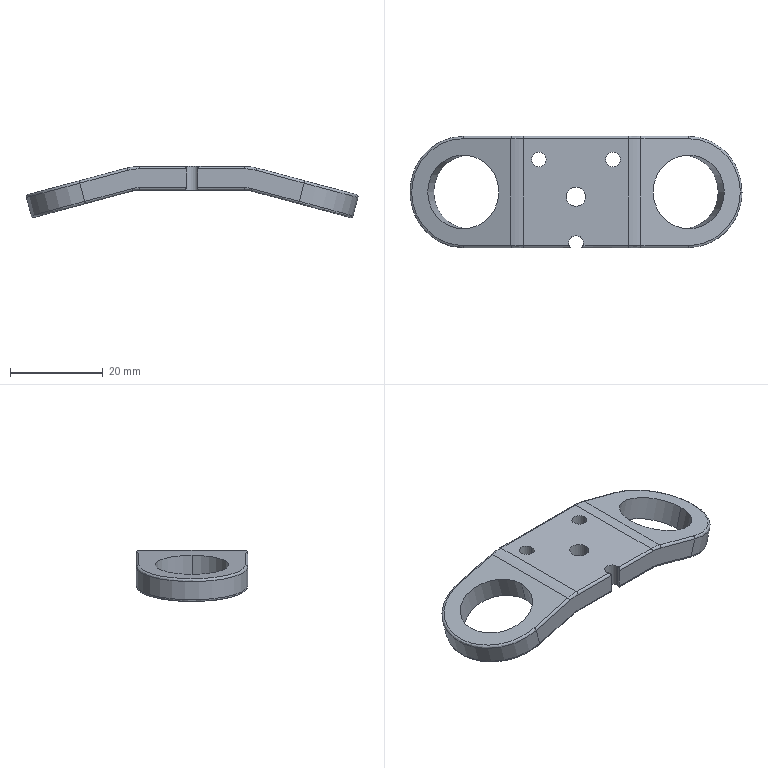Part | SolidWorks | features BaseBody 1 | 1 solid | 57 faces | box 71.498 x 24 x 10.999 mm | volume 5936 mm3 | cylinder 34 | spline 14 | plane 9 | commonest cylinder face diameters 1.016 x14 3.175 x7 15.875 x4 24 x3 4.166 x2 10.16 x2